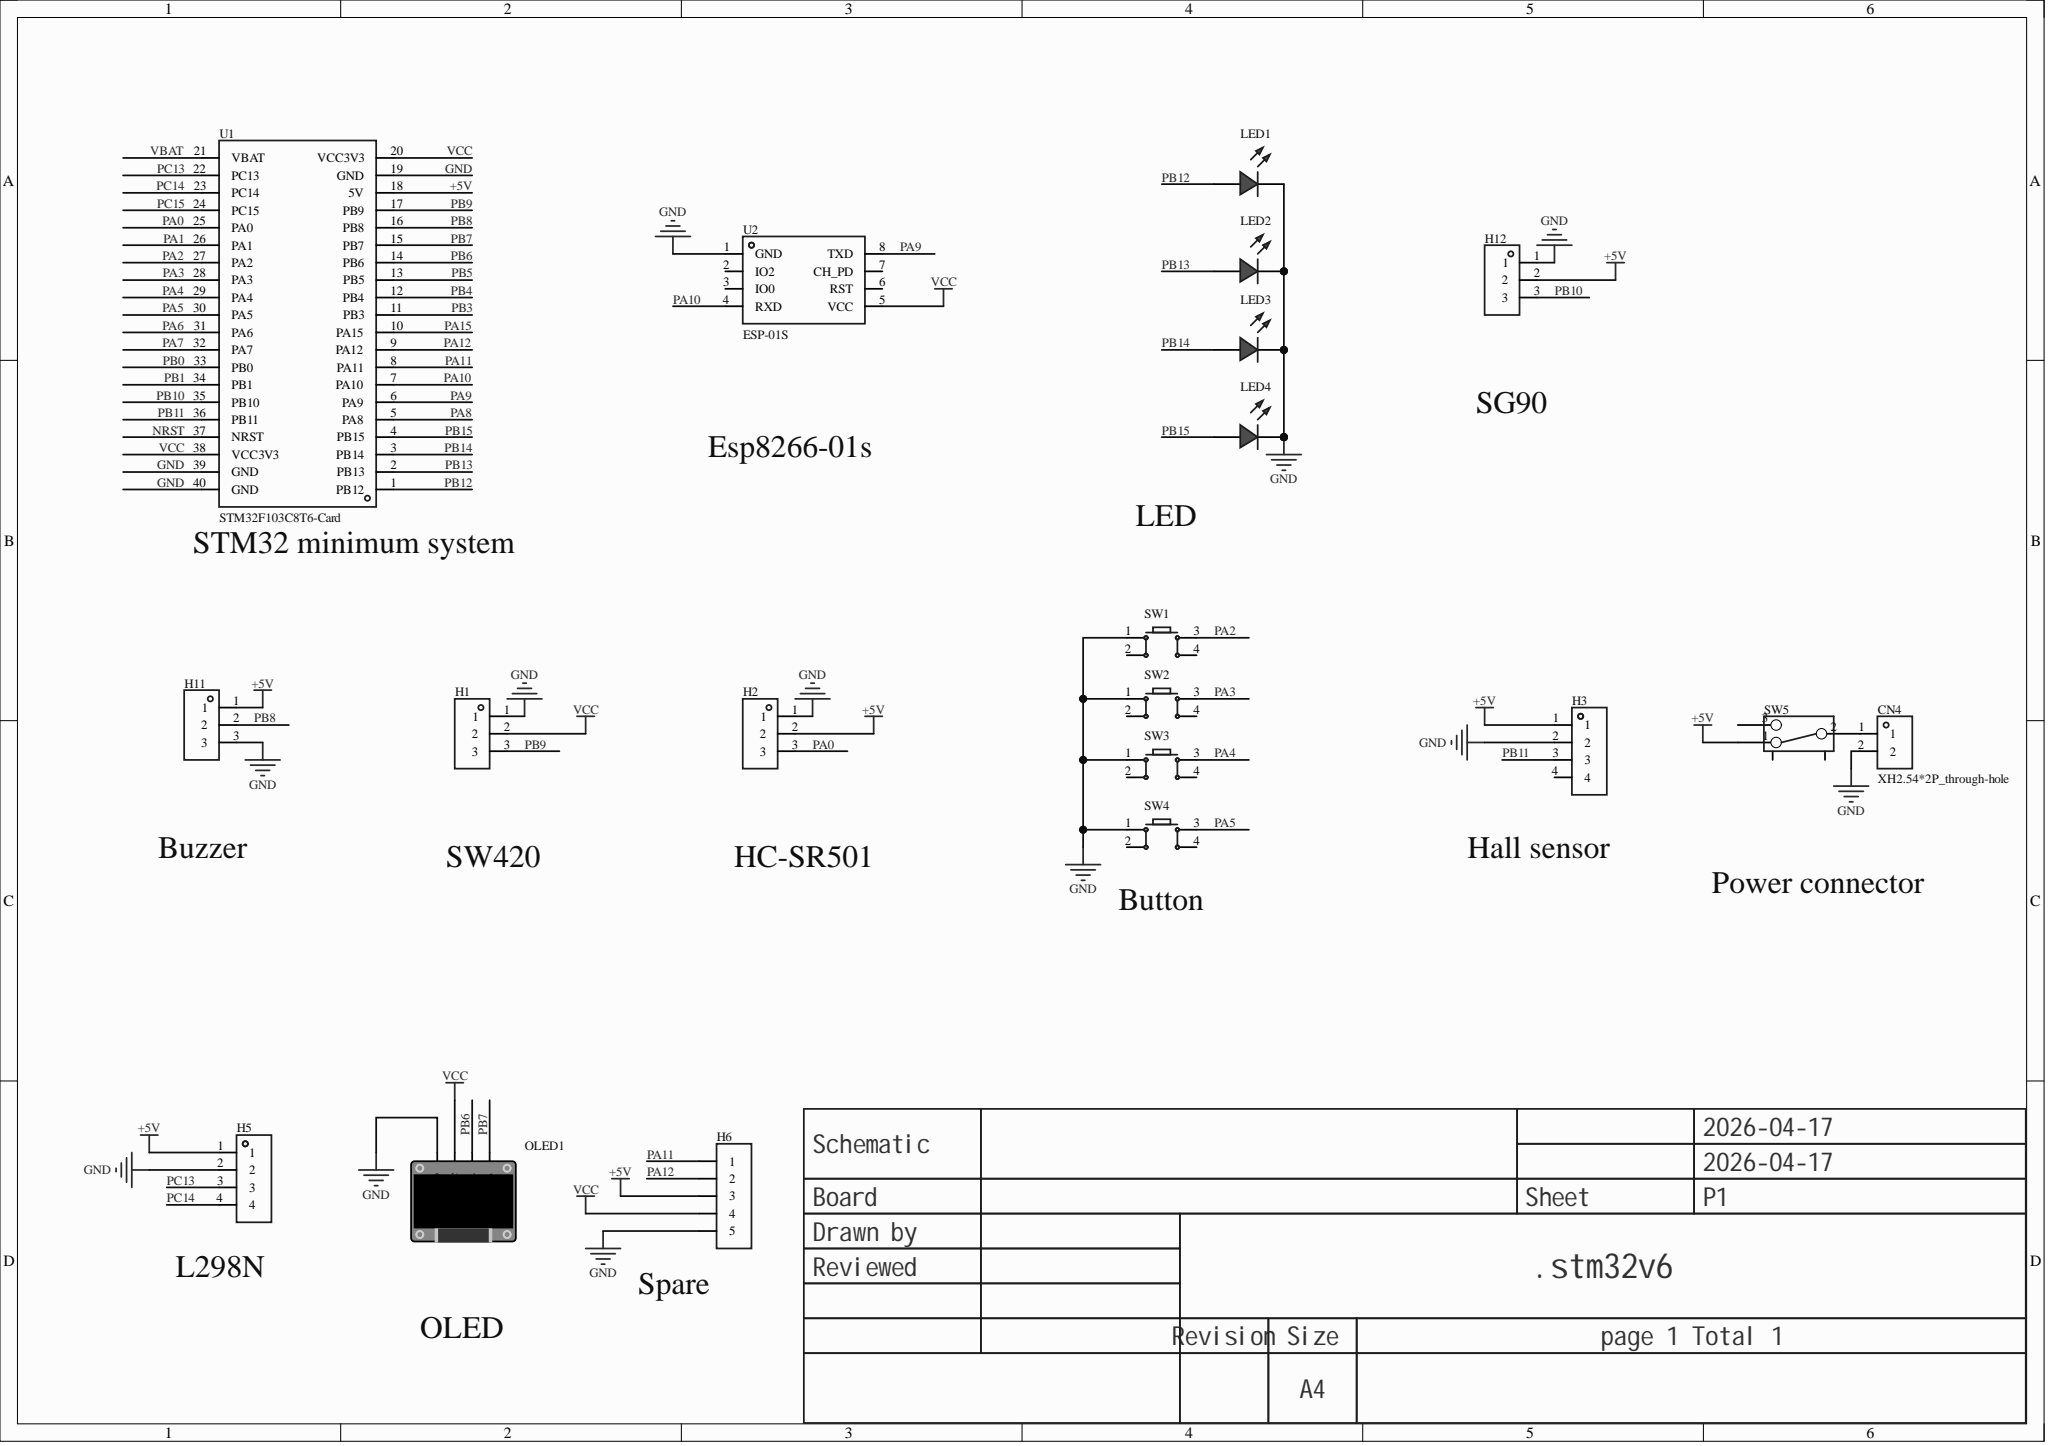Circuit board | Altium Designer | 20 parts | 25 nets
Bill of materials:
Comment,Description,Designator,Footprint,LibRef,Quantity
"XH2.54*2P_through-hole","","CN4","CONN-TH_2P-P2.50-XH2.54-2P","XH2.54*2P_直插","1"
"","","H1, H2, H11, H12","HDR-TH_3P-P2.54-V-F","HDR-F_2.54_1x3P","4"
"","","H3, H5","HDR-TH_4P-P2.54-V-F","HDR-F_2.54_1x4P","2"
"","","H6","HDR-TH_5P-P2.54-V-F","HDR-F_2.54_1x5P","1"
"","","LED1, LED2, LED3, LED4","LED-TH_5mm","LED_TH-R_5mm","4"
"","","OLED1","0.96OLED_4P","0.96OLED模块_4P","1"
"","","SW1, SW2, SW3, SW4","SW-TH_4P-L6.0-W6.0-P4.50-LS6.5","Key_TH_6x6x6","4"
"","","SW5","拨动开关","拨动开关_正","1"
"STM32F103C8T6-Card","","U1","CONN-TH_L53.3-W22.9_STM32F103C8T6-CARD","STM32F103C8T6-Card","1"
"ESP-01S","","U2","WIFIM-TH_ESP-01S","ESP-01S_C111009","1"
Netlist (Protel format):
[
CN4
CONN-TH_2P-P2.50-XH2.54-2P
XH2.54*2P_through-hole



]
[
H1
HDR-TH_3P-P2.54-V-F




]
[
H2
HDR-TH_3P-P2.54-V-F




]
[
H3
HDR-TH_4P-P2.54-V-F




]
[
H5
HDR-TH_4P-P2.54-V-F




]
[
H6
HDR-TH_5P-P2.54-V-F




]
[
H11
HDR-TH_3P-P2.54-V-F




]
[
H12
HDR-TH_3P-P2.54-V-F




]
[
LED1
LED-TH_5mm




]
[
LED2
LED-TH_5mm




]
[
LED3
LED-TH_5mm




]
[
LED4
LED-TH_5mm




]
[
OLED1
0.96OLED_4P




]
[
SW1
SW-TH_4P-L6.0-W6.0-P4.50-LS6.5




]
[
SW2
SW-TH_4P-L6.0-W6.0-P4.50-LS6.5




]
[
SW3
SW-TH_4P-L6.0-W6.0-P4.50-LS6.5




]
[
SW4
SW-TH_4P-L6.0-W6.0-P4.50-LS6.5




]
[
SW5
拨动开关




]
[
U1
CONN-TH_L53.3-W22.9_STM32F103C8T6-CARD
STM32F103C8T6-Card



]
[
U2
WIFIM-TH_ESP-01S
ESP-01S



]
(
VCC
H1-2
H6-4
OLED1-2
U1-20
U1-38
U2-5
)
(
PC14
H5-4
U1-23
)
(
PC13
H5-3
U1-22
)
(
PB15
LED4-1
U1-4
)
(
PB14
LED3-1
U1-3
)
(
PB13
LED2-1
U1-2
)
(
PB12
LED1-1
U1-1
)
(
PB11
H3-3
U1-36
)
(
PB10
H12-3
U1-35
)
(
PB9
H1-3
U1-17
)
(
PB8
H11-2
U1-16
)
(
PB7
OLED1-4
U1-15
)
(
PB6
OLED1-3
U1-14
)
(
PA12
H6-2
U1-9
)
(
PA11
H6-1
U1-8
)
(
PA10
U1-7
U2-4
)
(
PA9
U1-6
U2-8
)
(
PA5
SW4-3
U1-30
)
(
PA4
SW3-3
U1-29
)
(
PA3
SW2-3
U1-28
)
(
PA2
SW1-3
U1-27
)
(
PA0
H2-3
U1-25
)
(
NetCN4_1
CN4-1
SW5-2
)
(
GND
CN4-2
H1-1
H2-1
H3-2
H5-2
H6-5
H11-3
H12-1
LED1-2
LED2-2
LED3-2
LED4-2
OLED1-1
SW1-1
SW2-1
SW3-1
SW4-1
U1-19
U1-39
U1-40
U2-1
)
(
+5V
H2-2
H3-1
H5-1
H6-3
H11-1
H12-2
SW5-1
U1-18
)